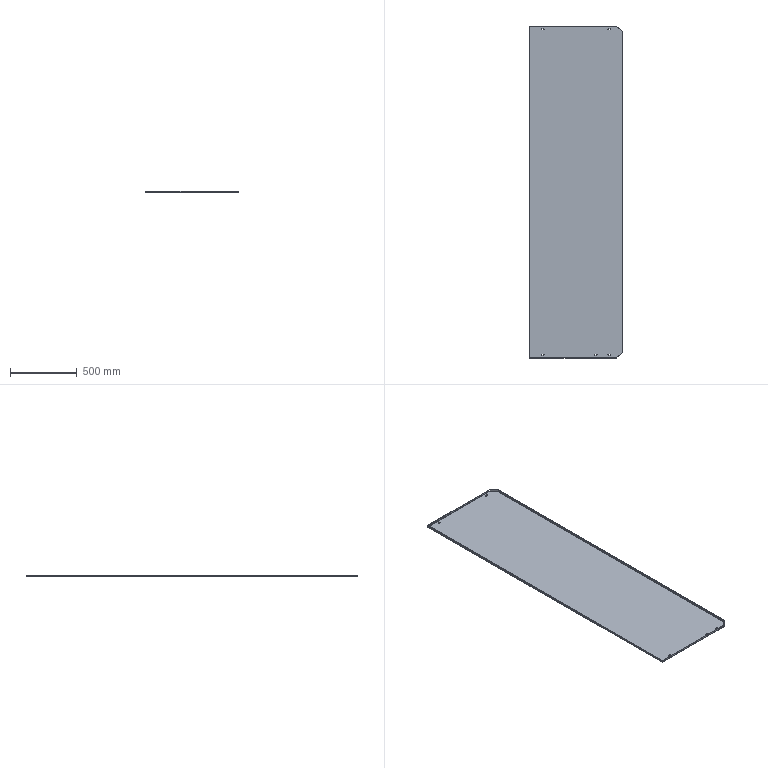Part | SolidWorks | features BaseBody 1 | 1 solid | 81 faces | box 702.5 x 2495 x 15 mm | volume 3654981 mm3 | plane 42 | cylinder 27 | spline 12 | commonest cylinder face diameters 7 x15 1.473 x6 5.473 x6